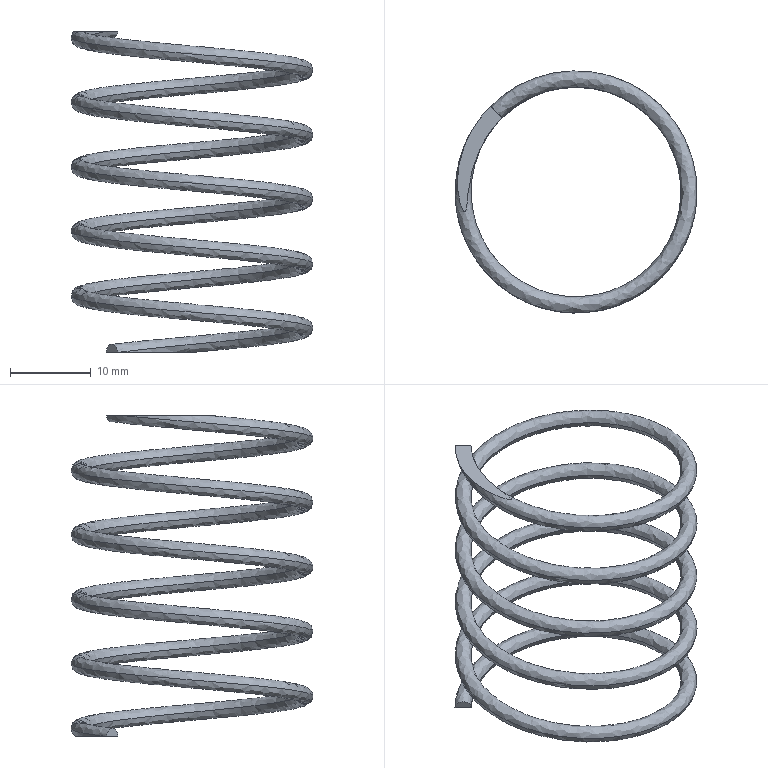Part | SolidWorks | features Helix 1, ICE 1, Sweep 1 | 1 solid | 6 faces | box 30 x 30 x 40 mm | volume 1368 mm3 | plane 4 | spline 2